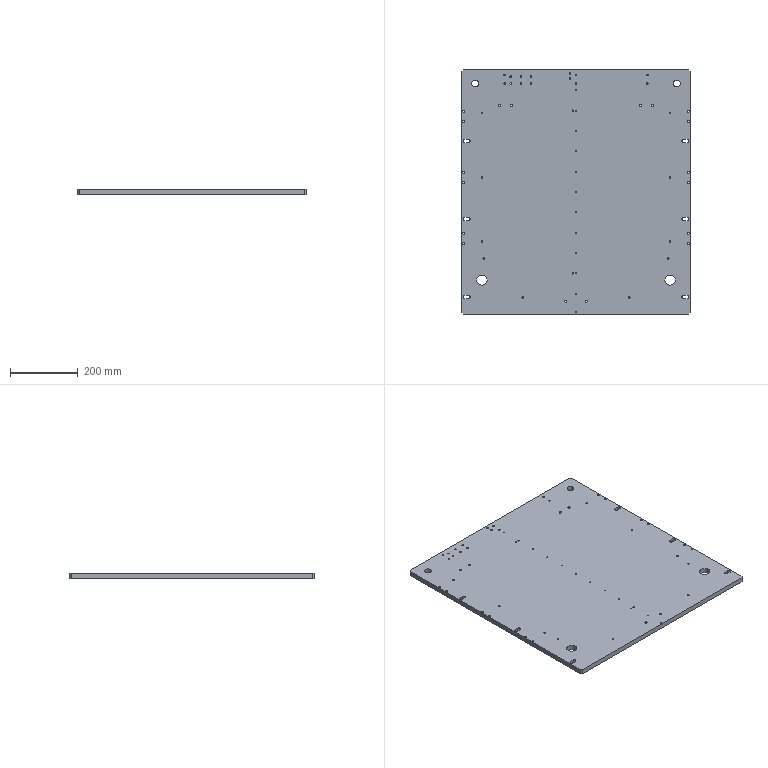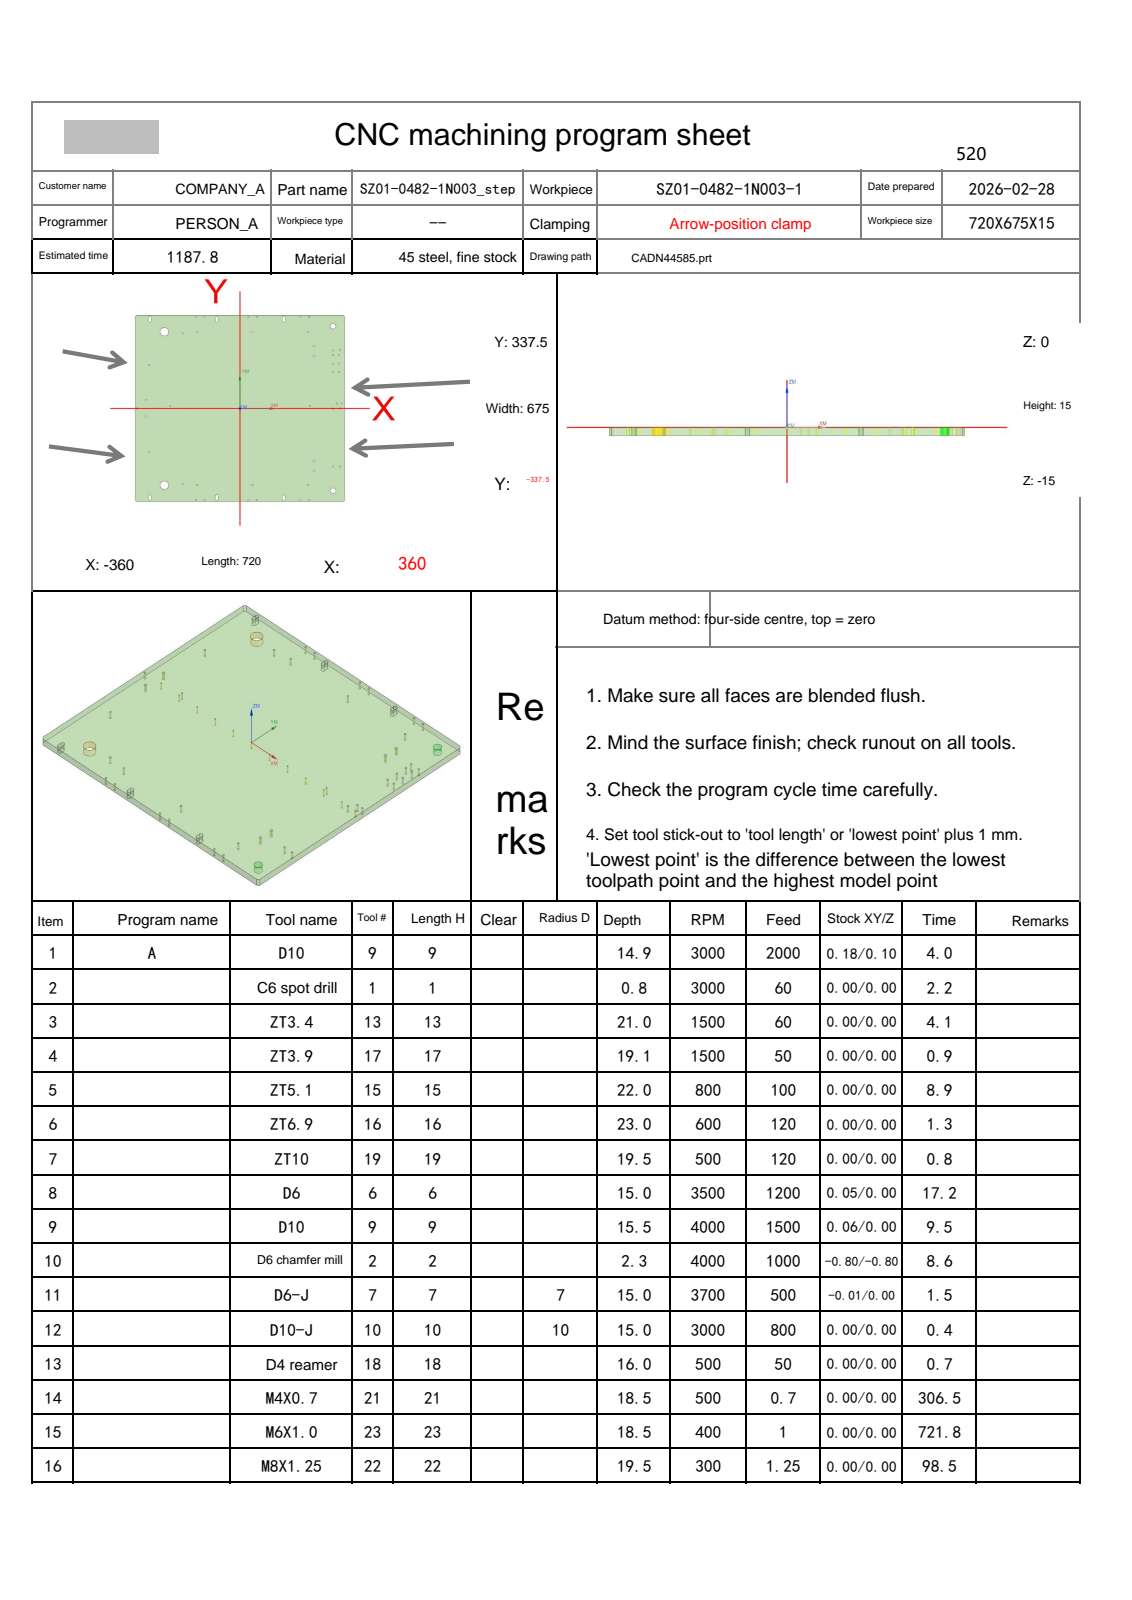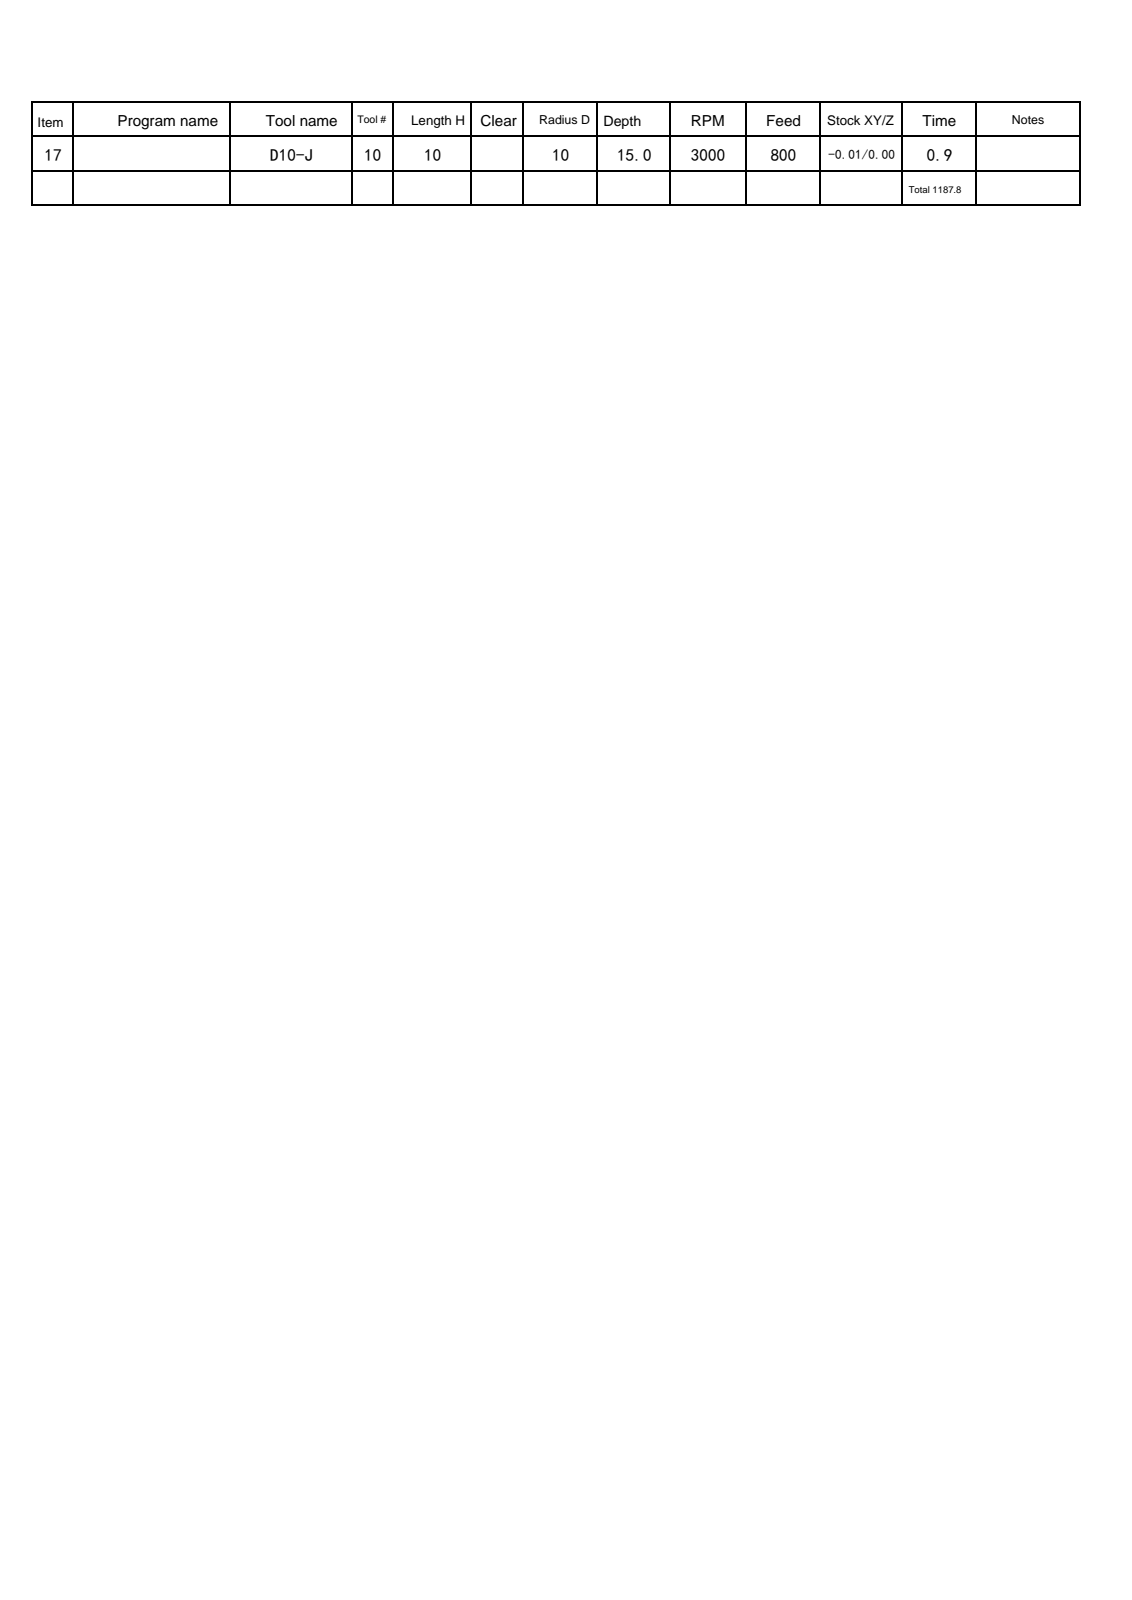NC program | NX | posted by the shop | part box 675 x 720 x 15 mm
Lines 1 to 1437 of 7907:
%
O0001
(Machine time: 2258.87 MIN)
(===Total Tool:15===)
(T9=D10     D=10.  R=0.   D-  H09 Z=-15.5 )
(T1=C6 spot drill   D=6.   R=0.   D-  H01 Z=-0.8  )
(T13=ZT3.4  D=3.4  DR_a=118 D-  H13 Z=-21.  )
(T17=ZT3.9  D=3.9  DR_a=120 D-  H17 Z=-19.13)
(T15=ZT5.1  D=5.1  DR_a=118 D-  H15 Z=-22.  )
(T16=ZT6.9  D=6.9  DR_a=120 D-  H16 Z=-23.  )
(T19=ZT10   D=10.  DR_a=118 D-  H19 Z=-19.5 )
(T6=D6      D=6.   R=0.   D-  H06 Z=-15.  )
(T2=D6 chamfer mill   D=6.   R=0.   D-  H02 Z=-2.3  )
(T7=D6-J    D=6.   R=0.   D7  H07 Z=-15.  )
(T10=D10-J  D=10.  R=0.   D10 H10 Z=-15.  )
(T18=D4 reamer   D=4.   DR_a=180 D-  H18 Z=-16.  )
(T21=M4X0.7 D=3.3  DR_a=180 D-  H21 Z=-18.5 )
(T23=M6X1.0 D=5.   DR_a=180 D-  H23 Z=-18.5 )
(T22=M8X1.25 D=6.8  DR_a=180 D-  H22 Z=-19.5 )
G80 G90 G17 G49 G40
G91 G28 Z0
M01
N1 T09 M06
(D10  D=10. R=0. H=09 ce=0.18 di=0.10)
G00 G90 G54 X352.299 Y347.527 M03 S3000
G43 H09 Z60.
M08
Z-.2
G01 X358.663 Y341.163 F2000.
X363.663 Y336.163
X370.027 Y329.799
G00 Z-.4
G01 X363.663 Y336.163
X358.663 Y341.163
X352.299 Y347.527
G00 Z-.6
G01 X358.663 Y341.163
X363.663 Y336.163
X370.027 Y329.799
G00 Z-.8
G01 X363.663 Y336.163
X358.663 Y341.163
X352.299 Y347.527
G00 Z-1.
G01 X358.663 Y341.163
X363.663 Y336.163
X370.027 Y329.799
G00 Z-1.2
G01 X363.663 Y336.163
X358.663 Y341.163
X352.299 Y347.527
G00 Z-1.4
G01 X358.663 Y341.163
X363.663 Y336.163
X370.027 Y329.799
G00 Z-1.6
G01 X363.663 Y336.163
X358.663 Y341.163
X352.299 Y347.527
G00 Z-1.8
G01 X358.663 Y341.163
X363.663 Y336.163
X370.027 Y329.799
G00 Z-2.
G01 X363.663 Y336.163
X358.663 Y341.163
X352.299 Y347.527
G00 Z-2.2
G01 X358.663 Y341.163
X363.663 Y336.163
X370.027 Y329.799
G00 Z-2.4
G01 X363.663 Y336.163
X358.663 Y341.163
X352.299 Y347.527
G00 Z-2.6
G01 X358.663 Y341.163
X363.663 Y336.163
X370.027 Y329.799
G00 Z-2.8
G01 X363.663 Y336.163
X358.663 Y341.163
X352.299 Y347.527
G00 Z-3.
G01 X358.663 Y341.163
X363.663 Y336.163
X370.027 Y329.799
G00 Z-3.2
G01 X363.663 Y336.163
X358.663 Y341.163
X352.299 Y347.527
G00 Z-3.4
G01 X358.663 Y341.163
X363.663 Y336.163
X370.027 Y329.799
G00 Z-3.6
G01 X363.663 Y336.163
X358.663 Y341.163
X352.299 Y347.527
G00 Z-3.8
G01 X358.663 Y341.163
X363.663 Y336.163
X370.027 Y329.799
G00 Z-4.
G01 X363.663 Y336.163
X358.663 Y341.163
X352.299 Y347.527
G00 Z-4.2
G01 X358.663 Y341.163
X363.663 Y336.163
X370.027 Y329.799
G00 Z-4.4
G01 X363.663 Y336.163
X358.663 Y341.163
X352.299 Y347.527
G00 Z-4.6
G01 X358.663 Y341.163
X363.663 Y336.163
X370.027 Y329.799
G00 Z-4.8
G01 X363.663 Y336.163
X358.663 Y341.163
X352.299 Y347.527
G00 Z-5.
G01 X358.663 Y341.163
X363.663 Y336.163
X370.027 Y329.799
G00 Z-5.2
G01 X363.663 Y336.163
X358.663 Y341.163
X352.299 Y347.527
G00 Z-5.4
G01 X358.663 Y341.163
X363.663 Y336.163
X370.027 Y329.799
G00 Z-5.6
G01 X363.663 Y336.163
X358.663 Y341.163
X352.299 Y347.527
G00 Z-5.8
G01 X358.663 Y341.163
X363.663 Y336.163
X370.027 Y329.799
G00 Z-6.
G01 X363.663 Y336.163
X358.663 Y341.163
X352.299 Y347.527
G00 Z-6.2
G01 X358.663 Y341.163
X363.663 Y336.163
X370.027 Y329.799
G00 Z-6.4
G01 X363.663 Y336.163
X358.663 Y341.163
X352.299 Y347.527
G00 Z-6.6
G01 X358.663 Y341.163
X363.663 Y336.163
X370.027 Y329.799
G00 Z-6.8
G01 X363.663 Y336.163
X358.663 Y341.163
X352.299 Y347.527
G00 Z-7.
G01 X358.663 Y341.163
X363.663 Y336.163
X370.027 Y329.799
G00 Z-7.2
G01 X363.663 Y336.163
X358.663 Y341.163
X352.299 Y347.527
G00 Z-7.4
G01 X358.663 Y341.163
X363.663 Y336.163
X370.027 Y329.799
G00 Z-7.6
G01 X363.663 Y336.163
X358.663 Y341.163
X352.299 Y347.527
G00 Z-7.8
G01 X358.663 Y341.163
X363.663 Y336.163
X370.027 Y329.799
G00 Z-8.
G01 X363.663 Y336.163
X358.663 Y341.163
X352.299 Y347.527
G00 Z-8.2
G01 X358.663 Y341.163
X363.663 Y336.163
X370.027 Y329.799
G00 Z-8.4
G01 X363.663 Y336.163
X358.663 Y341.163
X352.299 Y347.527
G00 Z-8.6
G01 X358.663 Y341.163
X363.663 Y336.163
X370.027 Y329.799
G00 Z-8.8
G01 X363.663 Y336.163
X358.663 Y341.163
X352.299 Y347.527
G00 Z-9.
G01 X358.663 Y341.163
X363.663 Y336.163
X370.027 Y329.799
G00 Z-9.2
G01 X363.663 Y336.163
X358.663 Y341.163
X352.299 Y347.527
G00 Z-9.4
G01 X358.663 Y341.163
X363.663 Y336.163
X370.027 Y329.799
G00 Z-9.6
G01 X363.663 Y336.163
X358.663 Y341.163
X352.299 Y347.527
G00 Z-9.8
G01 X358.663 Y341.163
X363.663 Y336.163
X370.027 Y329.799
G00 Z-10.
G01 X363.663 Y336.163
X358.663 Y341.163
X352.299 Y347.527
G00 Z-10.2
G01 X358.663 Y341.163
X363.663 Y336.163
X370.027 Y329.799
G00 Z-10.4
G01 X363.663 Y336.163
X358.663 Y341.163
X352.299 Y347.527
G00 Z-10.6
G01 X358.663 Y341.163
X363.663 Y336.163
X370.027 Y329.799
G00 Z-10.8
G01 X363.663 Y336.163
X358.663 Y341.163
X352.299 Y347.527
G00 Z-11.
G01 X358.663 Y341.163
X363.663 Y336.163
X370.027 Y329.799
G00 Z-11.2
G01 X363.663 Y336.163
X358.663 Y341.163
X352.299 Y347.527
G00 Z-11.4
G01 X358.663 Y341.163
X363.663 Y336.163
X370.027 Y329.799
G00 Z-11.6
G01 X363.663 Y336.163
X358.663 Y341.163
X352.299 Y347.527
G00 Z-11.8
G01 X358.663 Y341.163
X363.663 Y336.163
X370.027 Y329.799
G00 Z-12.
G01 X363.663 Y336.163
X358.663 Y341.163
X352.299 Y347.527
G00 Z-12.2
G01 X358.663 Y341.163
X363.663 Y336.163
X370.027 Y329.799
G00 Z-12.4
G01 X363.663 Y336.163
X358.663 Y341.163
X352.299 Y347.527
G00 Z-12.6
G01 X358.663 Y341.163
X363.663 Y336.163
X370.027 Y329.799
G00 Z-12.8
G01 X363.663 Y336.163
X358.663 Y341.163
X352.299 Y347.527
G00 Z-13.
G01 X358.663 Y341.163
X363.663 Y336.163
X370.027 Y329.799
G00 Z-13.2
G01 X363.663 Y336.163
X358.663 Y341.163
X352.299 Y347.527
G00 Z-13.4
G01 X358.663 Y341.163
X363.663 Y336.163
X370.027 Y329.799
G00 Z-13.6
G01 X363.663 Y336.163
X358.663 Y341.163
X352.299 Y347.527
G00 Z-13.8
G01 X358.663 Y341.163
X363.663 Y336.163
X370.027 Y329.799
G00 Z-14.
G01 X363.663 Y336.163
X358.663 Y341.163
X352.299 Y347.527
G00 Z-14.2
G01 X358.663 Y341.163
X363.663 Y336.163
X370.027 Y329.799
G00 Z-14.4
G01 X363.663 Y336.163
X358.663 Y341.163
X352.299 Y347.527
G00 Z-14.6
G01 X358.663 Y341.163
X363.663 Y336.163
X370.027 Y329.799
G00 Z-14.8
G01 X363.663 Y336.163
X358.663 Y341.163
X352.299 Y347.527
G00 Z-14.9
G01 X358.663 Y341.163
X363.663 Y336.163
X370.027 Y329.799
G00 Z60.
Y-329.799
Z-.2
G01 X363.663 Y-336.163
X358.663 Y-341.163
X352.299 Y-347.527
G00 Z-.4
G01 X358.663 Y-341.163
X363.663 Y-336.163
X370.027 Y-329.799
G00 Z-.6
G01 X363.663 Y-336.163
X358.663 Y-341.163
X352.299 Y-347.527
G00 Z-.8
G01 X358.663 Y-341.163
X363.663 Y-336.163
X370.027 Y-329.799
G00 Z-1.
G01 X363.663 Y-336.163
X358.663 Y-341.163
X352.299 Y-347.527
G00 Z-1.2
G01 X358.663 Y-341.163
X363.663 Y-336.163
X370.027 Y-329.799
G00 Z-1.4
G01 X363.663 Y-336.163
X358.663 Y-341.163
X352.299 Y-347.527
G00 Z-1.6
G01 X358.663 Y-341.163
X363.663 Y-336.163
X370.027 Y-329.799
G00 Z-1.8
G01 X363.663 Y-336.163
X358.663 Y-341.163
X352.299 Y-347.527
G00 Z-2.
G01 X358.663 Y-341.163
X363.663 Y-336.163
X370.027 Y-329.799
G00 Z-2.2
G01 X363.663 Y-336.163
X358.663 Y-341.163
X352.299 Y-347.527
G00 Z-2.4
G01 X358.663 Y-341.163
X363.663 Y-336.163
X370.027 Y-329.799
G00 Z-2.6
G01 X363.663 Y-336.163
X358.663 Y-341.163
X352.299 Y-347.527
G00 Z-2.8
G01 X358.663 Y-341.163
X363.663 Y-336.163
X370.027 Y-329.799
G00 Z-3.
G01 X363.663 Y-336.163
X358.663 Y-341.163
X352.299 Y-347.527
G00 Z-3.2
G01 X358.663 Y-341.163
X363.663 Y-336.163
X370.027 Y-329.799
G00 Z-3.4
G01 X363.663 Y-336.163
X358.663 Y-341.163
X352.299 Y-347.527
G00 Z-3.6
G01 X358.663 Y-341.163
X363.663 Y-336.163
X370.027 Y-329.799
G00 Z-3.8
G01 X363.663 Y-336.163
X358.663 Y-341.163
X352.299 Y-347.527
G00 Z-4.
G01 X358.663 Y-341.163
X363.663 Y-336.163
X370.027 Y-329.799
G00 Z-4.2
G01 X363.663 Y-336.163
X358.663 Y-341.163
X352.299 Y-347.527
G00 Z-4.4
G01 X358.663 Y-341.163
X363.663 Y-336.163
X370.027 Y-329.799
G00 Z-4.6
G01 X363.663 Y-336.163
X358.663 Y-341.163
X352.299 Y-347.527
G00 Z-4.8
G01 X358.663 Y-341.163
X363.663 Y-336.163
X370.027 Y-329.799
G00 Z-5.
G01 X363.663 Y-336.163
X358.663 Y-341.163
X352.299 Y-347.527
G00 Z-5.2
G01 X358.663 Y-341.163
X363.663 Y-336.163
X370.027 Y-329.799
G00 Z-5.4
G01 X363.663 Y-336.163
X358.663 Y-341.163
X352.299 Y-347.527
G00 Z-5.6
G01 X358.663 Y-341.163
X363.663 Y-336.163
X370.027 Y-329.799
G00 Z-5.8
G01 X363.663 Y-336.163
X358.663 Y-341.163
X352.299 Y-347.527
G00 Z-6.
G01 X358.663 Y-341.163
X363.663 Y-336.163
X370.027 Y-329.799
G00 Z-6.2
G01 X363.663 Y-336.163
X358.663 Y-341.163
X352.299 Y-347.527
G00 Z-6.4
G01 X358.663 Y-341.163
X363.663 Y-336.163
X370.027 Y-329.799
G00 Z-6.6
G01 X363.663 Y-336.163
X358.663 Y-341.163
X352.299 Y-347.527
G00 Z-6.8
G01 X358.663 Y-341.163
X363.663 Y-336.163
X370.027 Y-329.799
G00 Z-7.
G01 X363.663 Y-336.163
X358.663 Y-341.163
X352.299 Y-347.527
G00 Z-7.2
G01 X358.663 Y-341.163
X363.663 Y-336.163
X370.027 Y-329.799
G00 Z-7.4
G01 X363.663 Y-336.163
X358.663 Y-341.163
X352.299 Y-347.527
G00 Z-7.6
G01 X358.663 Y-341.163
X363.663 Y-336.163
X370.027 Y-329.799
G00 Z-7.8
G01 X363.663 Y-336.163
X358.663 Y-341.163
X352.299 Y-347.527
G00 Z-8.
G01 X358.663 Y-341.163
X363.663 Y-336.163
X370.027 Y-329.799
G00 Z-8.2
G01 X363.663 Y-336.163
X358.663 Y-341.163
X352.299 Y-347.527
G00 Z-8.4
G01 X358.663 Y-341.163
X363.663 Y-336.163
X370.027 Y-329.799
G00 Z-8.6
G01 X363.663 Y-336.163
X358.663 Y-341.163
X352.299 Y-347.527
G00 Z-8.8
G01 X358.663 Y-341.163
X363.663 Y-336.163
X370.027 Y-329.799
G00 Z-9.
G01 X363.663 Y-336.163
X358.663 Y-341.163
X352.299 Y-347.527
G00 Z-9.2
G01 X358.663 Y-341.163
X363.663 Y-336.163
X370.027 Y-329.799
G00 Z-9.4
G01 X363.663 Y-336.163
X358.663 Y-341.163
X352.299 Y-347.527
G00 Z-9.6
G01 X358.663 Y-341.163
X363.663 Y-336.163
X370.027 Y-329.799
G00 Z-9.8
G01 X363.663 Y-336.163
X358.663 Y-341.163
X352.299 Y-347.527
G00 Z-10.
G01 X358.663 Y-341.163
X363.663 Y-336.163
X370.027 Y-329.799
G00 Z-10.2
G01 X363.663 Y-336.163
X358.663 Y-341.163
X352.299 Y-347.527
G00 Z-10.4
G01 X358.663 Y-341.163
X363.663 Y-336.163
X370.027 Y-329.799
G00 Z-10.6
G01 X363.663 Y-336.163
X358.663 Y-341.163
X352.299 Y-347.527
G00 Z-10.8
G01 X358.663 Y-341.163
X363.663 Y-336.163
X370.027 Y-329.799
G00 Z-11.
G01 X363.663 Y-336.163
X358.663 Y-341.163
X352.299 Y-347.527
G00 Z-11.2
G01 X358.663 Y-341.163
X363.663 Y-336.163
X370.027 Y-329.799
G00 Z-11.4
G01 X363.663 Y-336.163
X358.663 Y-341.163
X352.299 Y-347.527
G00 Z-11.6
G01 X358.663 Y-341.163
X363.663 Y-336.163
X370.027 Y-329.799
G00 Z-11.8
G01 X363.663 Y-336.163
X358.663 Y-341.163
X352.299 Y-347.527
G00 Z-12.
G01 X358.663 Y-341.163
X363.663 Y-336.163
X370.027 Y-329.799
G00 Z-12.2
G01 X363.663 Y-336.163
X358.663 Y-341.163
X352.299 Y-347.527
G00 Z-12.4
G01 X358.663 Y-341.163
X363.663 Y-336.163
X370.027 Y-329.799
G00 Z-12.6
G01 X363.663 Y-336.163
X358.663 Y-341.163
X352.299 Y-347.527
G00 Z-12.8
G01 X358.663 Y-341.163
X363.663 Y-336.163
X370.027 Y-329.799
G00 Z-13.
G01 X363.663 Y-336.163
X358.663 Y-341.163
X352.299 Y-347.527
G00 Z-13.2
G01 X358.663 Y-341.163
X363.663 Y-336.163
X370.027 Y-329.799
G00 Z-13.4
G01 X363.663 Y-336.163
X358.663 Y-341.163
X352.299 Y-347.527
G00 Z-13.6
G01 X358.663 Y-341.163
X363.663 Y-336.163
X370.027 Y-329.799
G00 Z-13.8
G01 X363.663 Y-336.163
X358.663 Y-341.163
X352.299 Y-347.527
G00 Z-14.
G01 X358.663 Y-341.163
X363.663 Y-336.163
X370.027 Y-329.799
G00 Z-14.2
G01 X363.663 Y-336.163
X358.663 Y-341.163
X352.299 Y-347.527
G00 Z-14.4
G01 X358.663 Y-341.163
X363.663 Y-336.163
X370.027 Y-329.799
G00 Z-14.6
G01 X363.663 Y-336.163
X358.663 Y-341.163
X352.299 Y-347.527
G00 Z-14.8
G01 X358.663 Y-341.163
X363.663 Y-336.163
X370.027 Y-329.799
G00 Z-14.9
G01 X363.663 Y-336.163
X358.663 Y-341.163
X352.299 Y-347.527
G00 Z60.
X-352.299
Z-.2
G01 X-358.663 Y-341.163
X-363.663 Y-336.163
X-370.027 Y-329.799
G00 Z-.4
G01 X-363.663 Y-336.163
X-358.663 Y-341.163
X-352.299 Y-347.527
G00 Z-.6
G01 X-358.663 Y-341.163
X-363.663 Y-336.163
X-370.027 Y-329.799
G00 Z-.8
G01 X-363.663 Y-336.163
X-358.663 Y-341.163
X-352.299 Y-347.527
G00 Z-1.
G01 X-358.663 Y-341.163
X-363.663 Y-336.163
X-370.027 Y-329.799
G00 Z-1.2
G01 X-363.663 Y-336.163
X-358.663 Y-341.163
X-352.299 Y-347.527
G00 Z-1.4
G01 X-358.663 Y-341.163
X-363.663 Y-336.163
X-370.027 Y-329.799
G00 Z-1.6
G01 X-363.663 Y-336.163
X-358.663 Y-341.163
X-352.299 Y-347.527
G00 Z-1.8
G01 X-358.663 Y-341.163
X-363.663 Y-336.163
X-370.027 Y-329.799
G00 Z-2.
G01 X-363.663 Y-336.163
X-358.663 Y-341.163
X-352.299 Y-347.527
G00 Z-2.2
G01 X-358.663 Y-341.163
X-363.663 Y-336.163
X-370.027 Y-329.799
G00 Z-2.4
G01 X-363.663 Y-336.163
X-358.663 Y-341.163
X-352.299 Y-347.527
G00 Z-2.6
G01 X-358.663 Y-341.163
X-363.663 Y-336.163
X-370.027 Y-329.799
G00 Z-2.8
G01 X-363.663 Y-336.163
X-358.663 Y-341.163
X-352.299 Y-347.527
G00 Z-3.
G01 X-358.663 Y-341.163
X-363.663 Y-336.163
X-370.027 Y-329.799
G00 Z-3.2
G01 X-363.663 Y-336.163
X-358.663 Y-341.163
X-352.299 Y-347.527
G00 Z-3.4
G01 X-358.663 Y-341.163
X-363.663 Y-336.163
X-370.027 Y-329.799
G00 Z-3.6
G01 X-363.663 Y-336.163
X-358.663 Y-341.163
X-352.299 Y-347.527
G00 Z-3.8
G01 X-358.663 Y-341.163
X-363.663 Y-336.163
X-370.027 Y-329.799
G00 Z-4.
G01 X-363.663 Y-336.163
X-358.663 Y-341.163
X-352.299 Y-347.527
G00 Z-4.2
G01 X-358.663 Y-341.163
X-363.663 Y-336.163
X-370.027 Y-329.799
G00 Z-4.4
G01 X-363.663 Y-336.163
X-358.663 Y-341.163
X-352.299 Y-347.527
G00 Z-4.6
G01 X-358.663 Y-341.163
X-363.663 Y-336.163
X-370.027 Y-329.799
G00 Z-4.8
G01 X-363.663 Y-336.163
X-358.663 Y-341.163
X-352.299 Y-347.527
G00 Z-5.
G01 X-358.663 Y-341.163
X-363.663 Y-336.163
X-370.027 Y-329.799
G00 Z-5.2
G01 X-363.663 Y-336.163
X-358.663 Y-341.163
X-352.299 Y-347.527
G00 Z-5.4
G01 X-358.663 Y-341.163
X-363.663 Y-336.163
X-370.027 Y-329.799
G00 Z-5.6
G01 X-363.663 Y-336.163
X-358.663 Y-341.163
X-352.299 Y-347.527
G00 Z-5.8
G01 X-358.663 Y-341.163
X-363.663 Y-336.163
X-370.027 Y-329.799
G00 Z-6.
G01 X-363.663 Y-336.163
X-358.663 Y-341.163
X-352.299 Y-347.527
G00 Z-6.2
G01 X-358.663 Y-341.163
X-363.663 Y-336.163
X-370.027 Y-329.799
G00 Z-6.4
G01 X-363.663 Y-336.163
X-358.663 Y-341.163
X-352.299 Y-347.527
G00 Z-6.6
G01 X-358.663 Y-341.163
X-363.663 Y-336.163
X-370.027 Y-329.799
G00 Z-6.8
G01 X-363.663 Y-336.163
X-358.663 Y-341.163
X-352.299 Y-347.527
G00 Z-7.
G01 X-358.663 Y-341.163
X-363.663 Y-336.163
X-370.027 Y-329.799
G00 Z-7.2
G01 X-363.663 Y-336.163
X-358.663 Y-341.163
X-352.299 Y-347.527
G00 Z-7.4
G01 X-358.663 Y-341.163
X-363.663 Y-336.163
X-370.027 Y-329.799
G00 Z-7.6
G01 X-363.663 Y-336.163
X-358.663 Y-341.163
X-352.299 Y-347.527
G00 Z-7.8
G01 X-358.663 Y-341.163
X-363.663 Y-336.163
X-370.027 Y-329.799
G00 Z-8.
G01 X-363.663 Y-336.163
X-358.663 Y-341.163
X-352.299 Y-347.527
G00 Z-8.2
G01 X-358.663 Y-341.163
X-363.663 Y-336.163
X-370.027 Y-329.799
G00 Z-8.4
G01 X-363.663 Y-336.163
X-358.663 Y-341.163
X-352.299 Y-347.527
G00 Z-8.6
G01 X-358.663 Y-341.163
X-363.663 Y-336.163
X-370.027 Y-329.799
G00 Z-8.8
G01 X-363.663 Y-336.163
X-358.663 Y-341.163
X-352.299 Y-347.527
G00 Z-9.
G01 X-358.663 Y-341.163
X-363.663 Y-336.163
X-370.027 Y-329.799
G00 Z-9.2
G01 X-363.663 Y-336.163
X-358.663 Y-341.163
X-352.299 Y-347.527
G00 Z-9.4
G01 X-358.663 Y-341.163
X-363.663 Y-336.163
X-370.027 Y-329.799
G00 Z-9.6
G01 X-363.663 Y-336.163
X-358.663 Y-341.163
X-352.299 Y-347.527
G00 Z-9.8
G01 X-358.663 Y-341.163
X-363.663 Y-336.163
X-370.027 Y-329.799
G00 Z-10.
G01 X-363.663 Y-336.163
X-358.663 Y-341.163
X-352.299 Y-347.527
G00 Z-10.2
G01 X-358.663 Y-341.163
X-363.663 Y-336.163
X-370.027 Y-329.799
G00 Z-10.4
G01 X-363.663 Y-336.163
X-358.663 Y-341.163
X-352.299 Y-347.527
G00 Z-10.6
G01 X-358.663 Y-341.163
X-363.663 Y-336.163
X-370.027 Y-329.799
G00 Z-10.8
G01 X-363.663 Y-336.163
X-358.663 Y-341.163
X-352.299 Y-347.527
G00 Z-11.
G01 X-358.663 Y-341.163
X-363.663 Y-336.163
X-370.027 Y-329.799
G00 Z-11.2
G01 X-363.663 Y-336.163
X-358.663 Y-341.163
X-352.299 Y-347.527
G00 Z-11.4
G01 X-358.663 Y-341.163
X-363.663 Y-336.163
X-370.027 Y-329.799
G00 Z-11.6
G01 X-363.663 Y-336.163
X-358.663 Y-341.163
X-352.299 Y-347.527
G00 Z-11.8
G01 X-358.663 Y-341.163
X-363.663 Y-336.163
X-370.027 Y-329.799
G00 Z-12.
G01 X-363.663 Y-336.163
X-358.663 Y-341.163
X-352.299 Y-347.527
G00 Z-12.2
G01 X-358.663 Y-341.163
X-363.663 Y-336.163
X-370.027 Y-329.799
G00 Z-12.4
G01 X-363.663 Y-336.163
X-358.663 Y-341.163
X-352.299 Y-347.527
G00 Z-12.6
G01 X-358.663 Y-341.163
X-363.663 Y-336.163
X-370.027 Y-329.799
G00 Z-12.8
G01 X-363.663 Y-336.163
X-358.663 Y-341.163
X-352.299 Y-347.527
G00 Z-13.
G01 X-358.663 Y-341.163
X-363.663 Y-336.163
X-370.027 Y-329.799
G00 Z-13.2
G01 X-363.663 Y-336.163
X-358.663 Y-341.163
X-352.299 Y-347.527
G00 Z-13.4
G01 X-358.663 Y-341.163
X-363.663 Y-336.163
X-370.027 Y-329.799
G00 Z-13.6
G01 X-363.663 Y-336.163
X-358.663 Y-341.163
X-352.299 Y-347.527
G00 Z-13.8
G01 X-358.663 Y-341.163
X-363.663 Y-336.163
X-370.027 Y-329.799
G00 Z-14.
G01 X-363.663 Y-336.163
X-358.663 Y-341.163
X-352.299 Y-347.527
G00 Z-14.2
G01 X-358.663 Y-341.163
X-363.663 Y-336.163
X-370.027 Y-329.799
G00 Z-14.4
G01 X-363.663 Y-336.163
X-358.663 Y-341.163
X-352.299 Y-347.527
G00 Z-14.6
G01 X-358.663 Y-341.163
X-363.663 Y-336.163
X-370.027 Y-329.799
G00 Z-14.8
G01 X-363.663 Y-336.163
X-358.663 Y-341.163
X-352.299 Y-347.527
G00 Z-14.9
G01 X-358.663 Y-341.163
X-363.663 Y-336.163
X-370.027 Y-329.799
G00 Z60.
Y329.799
Z-.2
G01 X-363.663 Y336.163
X-358.663 Y341.163
X-352.299 Y347.527
G00 Z-.4
G01 X-358.663 Y341.163
X-363.663 Y336.163
X-370.027 Y329.799
G00 Z-.6
G01 X-363.663 Y336.163
X-358.663 Y341.163
X-352.299 Y347.527
G00 Z-.8
G01 X-358.663 Y341.163
X-363.663 Y336.163
X-370.027 Y329.799
G00 Z-1.
G01 X-363.663 Y336.163
X-358.663 Y341.163
X-352.299 Y347.527
G00 Z-1.2
G01 X-358.663 Y341.163
X-363.663 Y336.163
X-370.027 Y329.799
G00 Z-1.4
G01 X-363.663 Y336.163
X-358.663 Y341.163
X-352.299 Y347.527
G00 Z-1.6
G01 X-358.663 Y341.163
X-363.663 Y336.163
X-370.027 Y329.799
G00 Z-1.8
G01 X-363.663 Y336.163
X-358.663 Y341.163
X-352.299 Y347.527
G00 Z-2.
G01 X-358.663 Y341.163
X-363.663 Y336.163
X-370.027 Y329.799
G00 Z-2.2
G01 X-363.663 Y336.163
X-358.663 Y341.163
X-352.299 Y347.527
G00 Z-2.4
G01 X-358.663 Y341.163
X-363.663 Y336.163
X-370.027 Y329.799
G00 Z-2.6
G01 X-363.663 Y336.163
X-358.663 Y341.163
X-352.299 Y347.527
G00 Z-2.8
G01 X-358.663 Y341.163
X-363.663 Y336.163
X-370.027 Y329.799
G00 Z-3.
G01 X-363.663 Y336.163
X-358.663 Y341.163
X-352.299 Y347.527
G00 Z-3.2
G01 X-358.663 Y341.163
X-363.663 Y336.163
X-370.027 Y329.799
G00 Z-3.4
G01 X-363.663 Y336.163
X-358.663 Y341.163
X-352.299 Y347.527
G00 Z-3.6
G01 X-358.663 Y341.163
X-363.663 Y336.163
X-370.027 Y329.799
G00 Z-3.8
G01 X-363.663 Y336.163
X-358.663 Y341.163
X-352.299 Y347.527
G00 Z-4.
G01 X-358.663 Y341.163
X-363.663 Y336.163
X-370.027 Y329.799
G00 Z-4.2
G01 X-363.663 Y336.163
X-358.663 Y341.163
X-352.299 Y347.527
G00 Z-4.4
G01 X-358.663 Y341.163
X-363.663 Y336.163
X-370.027 Y329.799
G00 Z-4.6
G01 X-363.663 Y336.163
X-358.663 Y341.163
X-352.299 Y347.527
G00 Z-4.8
G01 X-358.663 Y341.163
X-363.663 Y336.163
X-370.027 Y329.799
G00 Z-5.
G01 X-363.663 Y336.163
X-358.663 Y341.163
X-352.299 Y347.527
G00 Z-5.2
G01 X-358.663 Y341.163
X-363.663 Y336.163
X-370.027 Y329.799
G00 Z-5.4
G01 X-363.663 Y336.163
X-358.663 Y341.163
X-352.299 Y347.527
G00 Z-5.6
G01 X-358.663 Y341.163
X-363.663 Y336.163
X-370.027 Y329.799
G00 Z-5.8
G01 X-363.663 Y336.163
X-358.663 Y341.163
X-352.299 Y347.527
G00 Z-6.
G01 X-358.663 Y341.163
X-363.663 Y336.163
X-370.027 Y329.799
G00 Z-6.2
G01 X-363.663 Y336.163
X-358.663 Y341.163
X-352.299 Y347.527
G00 Z-6.4
G01 X-358.663 Y341.163
X-363.663 Y336.163
X-370.027 Y329.799
G00 Z-6.6
G01 X-363.663 Y336.163
X-358.663 Y341.163
X-352.299 Y347.527
G00 Z-6.8
G01 X-358.663 Y341.163
X-363.663 Y336.163
X-370.027 Y329.799
G00 Z-7.
G01 X-363.663 Y336.163
X-358.663 Y341.163
X-352.299 Y347.527
G00 Z-7.2
G01 X-358.663 Y341.163
X-363.663 Y336.163
X-370.027 Y329.799
G00 Z-7.4
G01 X-363.663 Y336.163
X-358.663 Y341.163
X-352.299 Y347.527
G00 Z-7.6
G01 X-358.663 Y341.163
X-363.663 Y336.163
X-370.027 Y329.799
G00 Z-7.8
G01 X-363.663 Y336.163
X-358.663 Y341.163
X-352.299 Y347.527
G00 Z-8.
G01 X-358.663 Y341.163
X-363.663 Y336.163
X-370.027 Y329.799
G00 Z-8.2
G01 X-363.663 Y336.163
X-358.663 Y341.163
X-352.299 Y347.527
G00 Z-8.4
G01 X-358.663 Y341.163
X-363.663 Y336.163
X-370.027 Y329.799
G00 Z-8.6
G01 X-363.663 Y336.163
X-358.663 Y341.163
X-352.299 Y347.527
G00 Z-8.8
G01 X-358.663 Y341.163
X-363.663 Y336.163
X-370.027 Y329.799
G00 Z-9.
G01 X-363.663 Y336.163
X-358.663 Y341.163
X-352.299 Y347.527
G00 Z-9.2
G01 X-358.663 Y341.163
X-363.663 Y336.163
X-370.027 Y329.799
G00 Z-9.4
G01 X-363.663 Y336.163
X-358.663 Y341.163
X-352.299 Y347.527
G00 Z-9.6
G01 X-358.663 Y341.163
X-363.663 Y336.163
X-370.027 Y329.799
G00 Z-9.8
G01 X-363.663 Y336.163
X-358.663 Y341.163
X-352.299 Y347.527
G00 Z-10.
G01 X-358.663 Y341.163
X-363.663 Y336.163
X-370.027 Y329.799
G00 Z-10.2
G01 X-363.663 Y336.163
X-358.663 Y341.163
X-352.299 Y347.527
G00 Z-10.4
G01 X-358.663 Y341.163
X-363.663 Y336.163
X-370.027 Y329.799
G00 Z-10.6
G01 X-363.663 Y336.163
X-358.663 Y341.163
X-352.299 Y347.527
G00 Z-10.8
G01 X-358.663 Y341.163
X-363.663 Y336.163
X-370.027 Y329.799
G00 Z-11.
G01 X-363.663 Y336.163
X-358.663 Y341.163
X-352.299 Y347.527
G00 Z-11.2
G01 X-358.663 Y341.163
X-363.663 Y336.163
X-370.027 Y329.799
G00 Z-11.4
G01 X-363.663 Y336.163
X-358.663 Y341.163
X-352.299 Y347.527
G00 Z-11.6
G01 X-358.663 Y341.163
X-363.663 Y336.163
X-370.027 Y329.799
G00 Z-11.8
G01 X-363.663 Y336.163
X-358.663 Y341.163
X-352.299 Y347.527
G00 Z-12.
G01 X-358.663 Y341.163
X-363.663 Y336.163
X-370.027 Y329.799
G00 Z-12.2
G01 X-363.663 Y336.163
X-358.663 Y341.163
X-352.299 Y347.527
G00 Z-12.4
G01 X-358.663 Y341.163
X-363.663 Y336.163
X-370.027 Y329.799
G00 Z-12.6
G01 X-363.663 Y336.163
X-358.663 Y341.163
X-352.299 Y347.527
G00 Z-12.8
G01 X-358.663 Y341.163
X-363.663 Y336.163
X-370.027 Y329.799
G00 Z-13.
G01 X-363.663 Y336.163
X-358.663 Y341.163
X-352.299 Y347.527
G00 Z-13.2
G01 X-358.663 Y341.163
X-363.663 Y336.163
X-370.027 Y329.799
G00 Z-13.4
G01 X-363.663 Y336.163
X-358.663 Y341.163
X-352.299 Y347.527
G00 Z-13.6
G01 X-358.663 Y341.163
X-363.663 Y336.163
X-370.027 Y329.799
G00 Z-13.8
G01 X-363.663 Y336.163
X-358.663 Y341.163
X-352.299 Y347.527
G00 Z-14.
G01 X-358.663 Y341.163
X-363.663 Y336.163
X-370.027 Y329.799
G00 Z-14.2
G01 X-363.663 Y336.163
X-358.663 Y341.163
X-352.299 Y347.527
G00 Z-14.4
G01 X-358.663 Y341.163
X-363.663 Y336.163
X-370.027 Y329.799
G00 Z-14.6
G01 X-363.663 Y336.163
X-358.663 Y341.163
X-352.299 Y347.527
G00 Z-14.8
G01 X-358.663 Y341.163
X-363.663 Y336.163
X-370.027 Y329.799
G00 Z-14.9
G01 X-363.663 Y336.163
X-358.663 Y341.163
X-352.299 Y347.527
G00 Z60.
G91 G28 Z0.0
M05
M09
G91 G28 Z0.0
M01
N2 T01 M06
(C6 spot drill  D=6. R=0. H=01 ce=0.00 di=0.10)
G00 G90 G54 X320. Y-297.5 M03 S3000
G43 H01 Z30.
M08
G98 G81 X320. Y-297.5 Z-.8 R1. F60.
X345. Y-210.
X320.
X255. Y-189.5
Y-225.5
X233. Y-277.
X238. Y-331.5
X208.
X58.
X28.
X43. Y-277.
X-122. Y-331.5
X-152.
X-147. Y-277.
X-197. Y-271.932
X-260. Y-277.5
X-311.932 Y-157.
X-322. Y-30.
X-354. Y0.0
X-322. Y30.
X-300. Y0.0
X-240. Y9.5
Y0.0
X-180.
X-120.
X-60.
X0.0
X60.
X120.
X180.
X240.
Y9.5
X300. Y0.0
X320.
X345.
X350. Y18.
X334.
X340. Y132.5
X320.
Y162.5
X340.
Y192.5
X345. Y210.
X320.
Y192.5
X255. Y189.5
Y225.5
X233. Y277.
X320. Y297.5
X238. Y331.5
X208.
X58.
X28.
X43. Y277.
X-122. Y331.5
X-152.
X-147. Y277.
X-197. Y271.932
X-260. Y277.5
X-311.932 Y157.
G80
G00 Z30.
G91 G28 Z0.0
M05
M09
G91 G28 Z0.0
M01
N3 T13 M06
(ZT3.4 D=3.4 DR_a=118 H=13)
G00 G90 G54 X-300. Y0.0 M03 S1500
G43 H13 Z30.
M08
G98 G83 X-300. Y0.0 Z-21. R1. F60. Q1.
X-240.
X-180.
X-120.
X-60.
X0.0
X60.
X120.
X180.
X240.
X300.
G80
G00 Z30.
G91 G28 Z0.0
M05
M09
G91 G28 Z0.0
M01
N4 T17 M06
(ZT3.9 D=3.9 DR_a=120 H=17)
G00 G90 G54 X240. Y9.5 M03 S1500
G43 H17 Z30.
M08
G98 G83 X240. Y9.5 Z-19.126 R1. F50. Q1.
X-240.
G80
G00 Z30.
G91 G28 Z0.0
M05
M09
G91 G28 Z0.0
M01
N5 T15 M06
(ZT5.1 D=5.1 DR_a=118 H=15)
G00 G90 G54 X320. Y0.0 M03 S800
G43 H15 Z30.
M08
G98 G83 X320. Y0.0 Z-22. R1. F100. Q2.
X345.
X350. Y18.
X334.
X340. Y132.5
X320.
Y162.5
X340.
Y192.5
X345. Y210.
X320. Y192.5
Y210.
X233. Y277.
X238. Y331.5
X208.
X58.
X28.
X43. Y277.
X-122. Y331.5
X-152.
X-147. Y277.
X-197. Y271.932
X-311.932 Y157.
X-354. Y0.0
X-311.932 Y-157.
X-197. Y-271.932
X-147. Y-277.
X-152. Y-331.5
X-122.
X43. Y-277.
X28. Y-331.5
X58.
X208.
X238.
X233. Y-277.
X320. Y-210.
X345.
G80
G00 Z30.
G91 G28 Z0.0
M05
M09
G91 G28 Z0.0
M01
N6 T16 M06
(ZT6.9 D=6.9 DR_a=120 H=16)
G00 G90 G54 X255. Y225.5 M03 S600
G43 H16 Z30.
M08
G98 G83 X255. Y225.5 Z-23. R1. F120. Q2.
Y189.5
Y-189.5
Y-225.5
X-322. Y-30.
Y30.
G80
G00 Z30.
G91 G28 Z0.0
M05
M09
G91 G28 Z0.0
M01
N7 T19 M06
(ZT10 D=10. DR_a=118 H=19)
G00 G90 G54 X320. Y-297.5 M03 S500
G43 H19 Z30.
M08
G98 G83 X320. Y-297.5 Z-19.504 R1. F120. Q2.
Y297.5
G80
G00 Z30.
G00 G90 X-260. Y-277.5 M03 S500
Z30.
G98 G83 X-260. Y-277.5 Z-19.004 R1. F120. Q2.
Y277.5
G80
G00 Z30.
G91 G28 Z0.0
M05
M09
G91 G28 Z0.0
M01